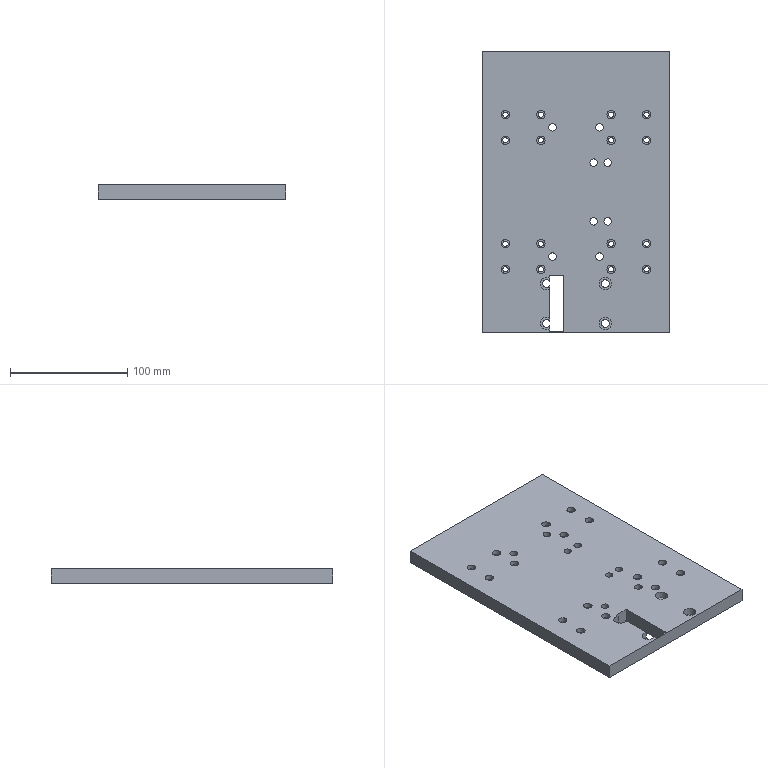Part | SolidWorks | features BaseBody 1 | 1 solid | 124 faces | box 160 x 240 x 12 mm | volume 443434 mm3 | cylinder 92 | plane 32 | commonest cylinder face diameters 4.5 x32 7.2 x32 6.5 x14 6.3 x8 10.6 x6